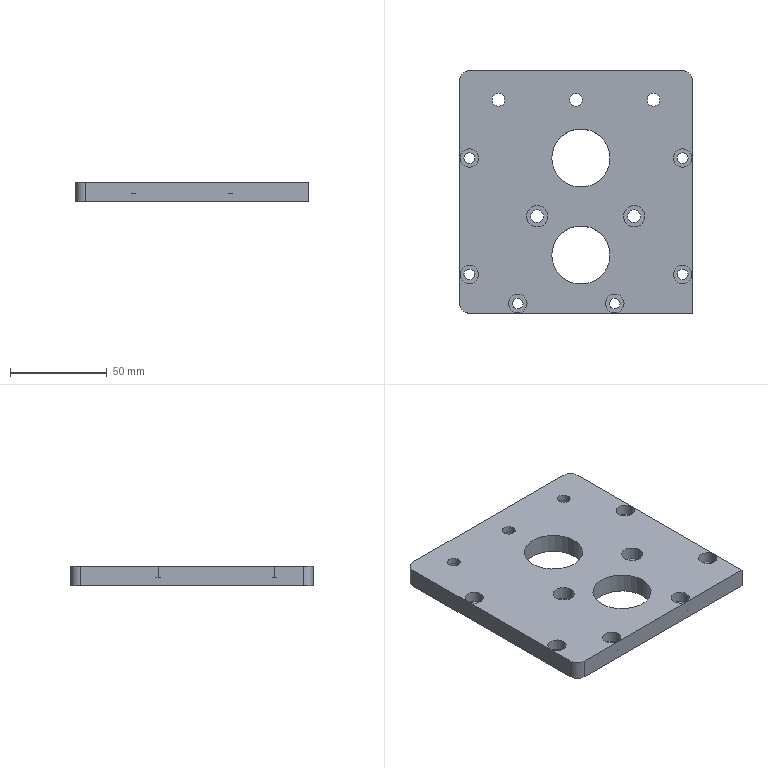Part | SolidWorks | features HoleWzd 4, Fillet 2, ICE 2, Extrusion 1, MirrorPattern 1 | 1 solid | 68 faces | box 120 x 125 x 10 mm | volume 128886 mm3 | cylinder 51 | plane 17 | commonest cylinder face diameters 5.5 x12 9.5 x12 6.6 x10 11 x10 30 x4 10 x3